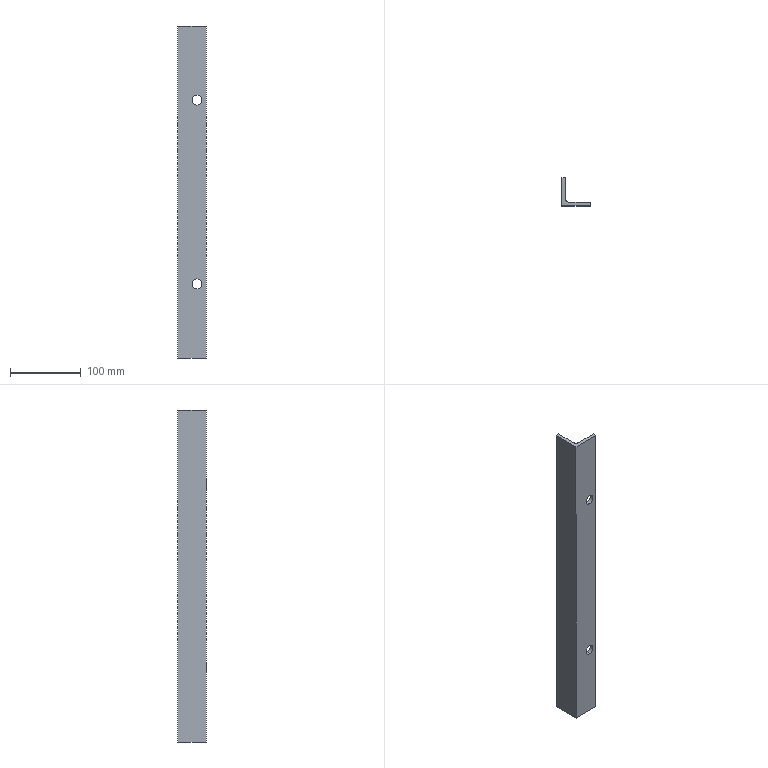Part | NX | features BREP 1 | 1 solid | 13 faces | box 40 x 40 x 470 mm | volume 177232 mm3 | plane 8 | cylinder 5 | commonest cylinder face diameters 14 x4 10 x1
STEP:
#1=CARTESIAN_POINT('',(27.,0.,-137.));
#2=VERTEX_POINT('',#1);
#3=CARTESIAN_POINT('',(27.,0.,-123.));
#4=VERTEX_POINT('',#3);
#5=CARTESIAN_POINT('',(27.,0.,-130.));
#6=DIRECTION('',(0.,1.,0.));
#7=DIRECTION('',(0.,0.,1.));
#8=AXIS2_PLACEMENT_3D('',#5,#6,#7);
#9=CIRCLE('',#8,7.);
#10=EDGE_CURVE('',#2,#4,#9,.T.);
#11=ORIENTED_EDGE('',*,*,#10,.F.);
#12=CARTESIAN_POINT('',(27.,5.,-137.));
#13=VERTEX_POINT('',#12);
#14=CARTESIAN_POINT('',(27.,0.,-137.));
#15=DIRECTION('',(0.,1.,0.));
#16=VECTOR('',#15,1000.);
#17=LINE('',#14,#16);
#18=EDGE_CURVE('',#2,#13,#17,.T.);
#19=ORIENTED_EDGE('',*,*,#18,.T.);
#20=CARTESIAN_POINT('',(27.,5.,-123.));
#21=VERTEX_POINT('',#20);
#22=CARTESIAN_POINT('',(27.,5.,-130.));
#23=DIRECTION('',(0.,1.,0.));
#24=DIRECTION('',(0.,0.,1.));
#25=AXIS2_PLACEMENT_3D('',#22,#23,#24);
#26=CIRCLE('',#25,7.);
#27=EDGE_CURVE('',#13,#21,#26,.T.);
#28=ORIENTED_EDGE('',*,*,#27,.T.);
#29=CARTESIAN_POINT('',(27.,0.,-123.));
#30=DIRECTION('',(0.,1.,0.));
#31=VECTOR('',#30,1000.);
#32=LINE('',#29,#31);
#33=EDGE_CURVE('',#4,#21,#32,.T.);
#34=ORIENTED_EDGE('',*,*,#33,.F.);
#35=EDGE_LOOP('',(#11,#19,#28,#34));
#36=FACE_BOUND('',#35,.T.);
#37=CARTESIAN_POINT('',(27.,0.,-130.));
#38=DIRECTION('',(0.,1.,0.));
#39=DIRECTION('',(0.,0.,-1.));
#40=AXIS2_PLACEMENT_3D('',#37,#38,#39);
#41=CYLINDRICAL_SURFACE('',#40,7.);
#42=ADVANCED_FACE('',(#36),#41,.F.);
#43=CARTESIAN_POINT('',(27.,0.,123.));
#44=VERTEX_POINT('',#43);
#45=CARTESIAN_POINT('',(27.,0.,137.));
#46=VERTEX_POINT('',#45);
#47=CARTESIAN_POINT('',(27.,0.,130.));
#48=DIRECTION('',(0.,1.,0.));
#49=DIRECTION('',(0.,0.,1.));
#50=AXIS2_PLACEMENT_3D('',#47,#48,#49);
#51=CIRCLE('',#50,7.);
#52=EDGE_CURVE('',#44,#46,#51,.T.);
#53=ORIENTED_EDGE('',*,*,#52,.F.);
#54=CARTESIAN_POINT('',(27.,5.,123.));
#55=VERTEX_POINT('',#54);
#56=CARTESIAN_POINT('',(27.,0.,123.));
#57=DIRECTION('',(0.,1.,0.));
#58=VECTOR('',#57,1000.);
#59=LINE('',#56,#58);
#60=EDGE_CURVE('',#44,#55,#59,.T.);
#61=ORIENTED_EDGE('',*,*,#60,.T.);
#62=CARTESIAN_POINT('',(27.,5.,137.));
#63=VERTEX_POINT('',#62);
#64=CARTESIAN_POINT('',(27.,5.,130.));
#65=DIRECTION('',(0.,1.,0.));
#66=DIRECTION('',(0.,0.,1.));
#67=AXIS2_PLACEMENT_3D('',#64,#65,#66);
#68=CIRCLE('',#67,7.);
#69=EDGE_CURVE('',#55,#63,#68,.T.);
#70=ORIENTED_EDGE('',*,*,#69,.T.);
#71=CARTESIAN_POINT('',(27.,0.,137.));
#72=DIRECTION('',(0.,1.,0.));
#73=VECTOR('',#72,1000.);
#74=LINE('',#71,#73);
#75=EDGE_CURVE('',#46,#63,#74,.T.);
#76=ORIENTED_EDGE('',*,*,#75,.F.);
#77=EDGE_LOOP('',(#53,#61,#70,#76));
#78=FACE_BOUND('',#77,.T.);
#79=CARTESIAN_POINT('',(27.,0.,130.));
#80=DIRECTION('',(0.,1.,0.));
#81=DIRECTION('',(0.,0.,-1.));
#82=AXIS2_PLACEMENT_3D('',#79,#80,#81);
#83=CYLINDRICAL_SURFACE('',#82,7.);
#84=ADVANCED_FACE('',(#78),#83,.F.);
#85=CARTESIAN_POINT('',(40.,0.,-235.));
#86=VERTEX_POINT('',#85);
#87=CARTESIAN_POINT('',(40.,5.,-235.));
#88=VERTEX_POINT('',#87);
#89=CARTESIAN_POINT('',(40.,5.,-235.));
#90=DIRECTION('',(0.,1.,0.));
#91=VECTOR('',#90,1000.);
#92=LINE('',#89,#91);
#93=EDGE_CURVE('',#86,#88,#92,.T.);
#94=ORIENTED_EDGE('',*,*,#93,.T.);
#95=CARTESIAN_POINT('',(40.,5.,235.));
#96=VERTEX_POINT('',#95);
#97=CARTESIAN_POINT('',(40.,5.,235.));
#98=DIRECTION('',(0.,0.,-1.));
#99=VECTOR('',#98,1000.);
#100=LINE('',#97,#99);
#101=EDGE_CURVE('',#96,#88,#100,.T.);
#102=ORIENTED_EDGE('',*,*,#101,.F.);
#103=CARTESIAN_POINT('',(40.,0.,235.));
#104=VERTEX_POINT('',#103);
#105=CARTESIAN_POINT('',(40.,5.,235.));
#106=DIRECTION('',(0.,1.,0.));
#107=VECTOR('',#106,1000.);
#108=LINE('',#105,#107);
#109=EDGE_CURVE('',#104,#96,#108,.T.);
#110=ORIENTED_EDGE('',*,*,#109,.F.);
#111=CARTESIAN_POINT('',(40.,0.,235.));
#112=DIRECTION('',(0.,0.,-1.));
#113=VECTOR('',#112,1000.);
#114=LINE('',#111,#113);
#115=EDGE_CURVE('',#104,#86,#114,.T.);
#116=ORIENTED_EDGE('',*,*,#115,.T.);
#117=EDGE_LOOP('',(#94,#102,#110,#116));
#118=FACE_BOUND('',#117,.T.);
#119=CARTESIAN_POINT('',(40.,5.,235.));
#120=DIRECTION('',(-1.,0.,0.));
#121=DIRECTION('',(0.,0.,-1.));
#122=AXIS2_PLACEMENT_3D('',#119,#120,#121);
#123=PLANE('',#122);
#124=ADVANCED_FACE('',(#118),#123,.F.);
#125=CARTESIAN_POINT('',(27.,5.,-130.));
#126=DIRECTION('',(0.,1.,0.));
#127=DIRECTION('',(0.,0.,1.));
#128=AXIS2_PLACEMENT_3D('',#125,#126,#127);
#129=CIRCLE('',#128,7.);
#130=EDGE_CURVE('',#21,#13,#129,.T.);
#131=ORIENTED_EDGE('',*,*,#130,.F.);
#132=ORIENTED_EDGE('',*,*,#27,.F.);
#133=EDGE_LOOP('',(#131,#132));
#134=FACE_BOUND('',#133,.T.);
#135=CARTESIAN_POINT('',(27.,5.,130.));
#136=DIRECTION('',(0.,1.,0.));
#137=DIRECTION('',(0.,0.,1.));
#138=AXIS2_PLACEMENT_3D('',#135,#136,#137);
#139=CIRCLE('',#138,7.);
#140=EDGE_CURVE('',#63,#55,#139,.T.);
#141=ORIENTED_EDGE('',*,*,#140,.F.);
#142=ORIENTED_EDGE('',*,*,#69,.F.);
#143=EDGE_LOOP('',(#141,#142));
#144=FACE_BOUND('',#143,.T.);
#145=CARTESIAN_POINT('',(10.,5.,-235.));
#146=VERTEX_POINT('',#145);
#147=CARTESIAN_POINT('',(10.,5.,-235.));
#148=DIRECTION('',(-1.,0.,0.));
#149=VECTOR('',#148,1000.);
#150=LINE('',#147,#149);
#151=EDGE_CURVE('',#88,#146,#150,.T.);
#152=ORIENTED_EDGE('',*,*,#151,.T.);
#153=CARTESIAN_POINT('',(10.,5.,235.));
#154=VERTEX_POINT('',#153);
#155=CARTESIAN_POINT('',(10.,5.,235.));
#156=DIRECTION('',(0.,0.,-1.));
#157=VECTOR('',#156,1000.);
#158=LINE('',#155,#157);
#159=EDGE_CURVE('',#154,#146,#158,.T.);
#160=ORIENTED_EDGE('',*,*,#159,.F.);
#161=CARTESIAN_POINT('',(10.,5.,235.));
#162=DIRECTION('',(-1.,0.,0.));
#163=VECTOR('',#162,1000.);
#164=LINE('',#161,#163);
#165=EDGE_CURVE('',#96,#154,#164,.T.);
#166=ORIENTED_EDGE('',*,*,#165,.F.);
#167=ORIENTED_EDGE('',*,*,#101,.T.);
#168=EDGE_LOOP('',(#152,#160,#166,#167));
#169=FACE_BOUND('',#168,.T.);
#170=CARTESIAN_POINT('',(10.,5.,235.));
#171=DIRECTION('',(0.,-1.,0.));
#172=DIRECTION('',(0.,0.,1.));
#173=AXIS2_PLACEMENT_3D('',#170,#171,#172);
#174=PLANE('',#173);
#175=ADVANCED_FACE('',(#134,#144,#169),#174,.F.);
#176=CARTESIAN_POINT('',(5.,10.,-235.));
#177=VERTEX_POINT('',#176);
#178=CARTESIAN_POINT('',(10.,10.,-235.));
#179=DIRECTION('',(0.,0.,-1.));
#180=DIRECTION('',(1.,0.,0.));
#181=AXIS2_PLACEMENT_3D('',#178,#179,#180);
#182=CIRCLE('',#181,5.);
#183=EDGE_CURVE('',#146,#177,#182,.T.);
#184=ORIENTED_EDGE('',*,*,#183,.T.);
#185=CARTESIAN_POINT('',(5.,10.,235.));
#186=VERTEX_POINT('',#185);
#187=CARTESIAN_POINT('',(5.,10.,235.));
#188=DIRECTION('',(0.,0.,-1.));
#189=VECTOR('',#188,1000.);
#190=LINE('',#187,#189);
#191=EDGE_CURVE('',#186,#177,#190,.T.);
#192=ORIENTED_EDGE('',*,*,#191,.F.);
#193=CARTESIAN_POINT('',(10.,10.,235.));
#194=DIRECTION('',(0.,0.,-1.));
#195=DIRECTION('',(1.,0.,0.));
#196=AXIS2_PLACEMENT_3D('',#193,#194,#195);
#197=CIRCLE('',#196,5.);
#198=EDGE_CURVE('',#154,#186,#197,.T.);
#199=ORIENTED_EDGE('',*,*,#198,.F.);
#200=ORIENTED_EDGE('',*,*,#159,.T.);
#201=EDGE_LOOP('',(#184,#192,#199,#200));
#202=FACE_BOUND('',#201,.T.);
#203=CARTESIAN_POINT('',(10.,10.,235.));
#204=DIRECTION('',(0.,0.,-1.));
#205=DIRECTION('',(1.,0.,0.));
#206=AXIS2_PLACEMENT_3D('',#203,#204,#205);
#207=CYLINDRICAL_SURFACE('',#206,5.);
#208=ADVANCED_FACE('',(#202),#207,.F.);
#209=CARTESIAN_POINT('',(5.,40.,-235.));
#210=VERTEX_POINT('',#209);
#211=CARTESIAN_POINT('',(5.,40.,-235.));
#212=DIRECTION('',(0.,1.,0.));
#213=VECTOR('',#212,1000.);
#214=LINE('',#211,#213);
#215=EDGE_CURVE('',#177,#210,#214,.T.);
#216=ORIENTED_EDGE('',*,*,#215,.T.);
#217=CARTESIAN_POINT('',(5.,40.,235.));
#218=VERTEX_POINT('',#217);
#219=CARTESIAN_POINT('',(5.,40.,235.));
#220=DIRECTION('',(0.,0.,-1.));
#221=VECTOR('',#220,1000.);
#222=LINE('',#219,#221);
#223=EDGE_CURVE('',#218,#210,#222,.T.);
#224=ORIENTED_EDGE('',*,*,#223,.F.);
#225=CARTESIAN_POINT('',(5.,40.,235.));
#226=DIRECTION('',(0.,1.,0.));
#227=VECTOR('',#226,1000.);
#228=LINE('',#225,#227);
#229=EDGE_CURVE('',#186,#218,#228,.T.);
#230=ORIENTED_EDGE('',*,*,#229,.F.);
#231=ORIENTED_EDGE('',*,*,#191,.T.);
#232=EDGE_LOOP('',(#216,#224,#230,#231));
#233=FACE_BOUND('',#232,.T.);
#234=CARTESIAN_POINT('',(5.,40.,235.));
#235=DIRECTION('',(-1.,0.,0.));
#236=DIRECTION('',(0.,0.,-1.));
#237=AXIS2_PLACEMENT_3D('',#234,#235,#236);
#238=PLANE('',#237);
#239=ADVANCED_FACE('',(#233),#238,.F.);
#240=CARTESIAN_POINT('',(0.,40.,-235.));
#241=VERTEX_POINT('',#240);
#242=CARTESIAN_POINT('',(0.,40.,-235.));
#243=DIRECTION('',(-1.,0.,0.));
#244=VECTOR('',#243,1000.);
#245=LINE('',#242,#244);
#246=EDGE_CURVE('',#210,#241,#245,.T.);
#247=ORIENTED_EDGE('',*,*,#246,.T.);
#248=CARTESIAN_POINT('',(0.,40.,235.));
#249=VERTEX_POINT('',#248);
#250=CARTESIAN_POINT('',(0.,40.,235.));
#251=DIRECTION('',(0.,0.,-1.));
#252=VECTOR('',#251,1000.);
#253=LINE('',#250,#252);
#254=EDGE_CURVE('',#249,#241,#253,.T.);
#255=ORIENTED_EDGE('',*,*,#254,.F.);
#256=CARTESIAN_POINT('',(0.,40.,235.));
#257=DIRECTION('',(-1.,0.,0.));
#258=VECTOR('',#257,1000.);
#259=LINE('',#256,#258);
#260=EDGE_CURVE('',#218,#249,#259,.T.);
#261=ORIENTED_EDGE('',*,*,#260,.F.);
#262=ORIENTED_EDGE('',*,*,#223,.T.);
#263=EDGE_LOOP('',(#247,#255,#261,#262));
#264=FACE_BOUND('',#263,.T.);
#265=CARTESIAN_POINT('',(0.,40.,235.));
#266=DIRECTION('',(0.,-1.,0.));
#267=DIRECTION('',(0.,0.,1.));
#268=AXIS2_PLACEMENT_3D('',#265,#266,#267);
#269=PLANE('',#268);
#270=ADVANCED_FACE('',(#264),#269,.F.);
#271=CARTESIAN_POINT('',(0.,0.,-235.));
#272=VERTEX_POINT('',#271);
#273=CARTESIAN_POINT('',(0.,0.,-235.));
#274=DIRECTION('',(0.,-1.,0.));
#275=VECTOR('',#274,1000.);
#276=LINE('',#273,#275);
#277=EDGE_CURVE('',#241,#272,#276,.T.);
#278=ORIENTED_EDGE('',*,*,#277,.T.);
#279=CARTESIAN_POINT('',(0.,0.,235.));
#280=VERTEX_POINT('',#279);
#281=CARTESIAN_POINT('',(0.,0.,235.));
#282=DIRECTION('',(0.,0.,-1.));
#283=VECTOR('',#282,1000.);
#284=LINE('',#281,#283);
#285=EDGE_CURVE('',#280,#272,#284,.T.);
#286=ORIENTED_EDGE('',*,*,#285,.F.);
#287=CARTESIAN_POINT('',(0.,0.,235.));
#288=DIRECTION('',(0.,-1.,0.));
#289=VECTOR('',#288,1000.);
#290=LINE('',#287,#289);
#291=EDGE_CURVE('',#249,#280,#290,.T.);
#292=ORIENTED_EDGE('',*,*,#291,.F.);
#293=ORIENTED_EDGE('',*,*,#254,.T.);
#294=EDGE_LOOP('',(#278,#286,#292,#293));
#295=FACE_BOUND('',#294,.T.);
#296=CARTESIAN_POINT('',(0.,0.,235.));
#297=DIRECTION('',(1.,0.,0.));
#298=DIRECTION('',(0.,0.,1.));
#299=AXIS2_PLACEMENT_3D('',#296,#297,#298);
#300=PLANE('',#299);
#301=ADVANCED_FACE('',(#295),#300,.F.);
#302=CARTESIAN_POINT('',(27.,0.,-130.));
#303=DIRECTION('',(0.,1.,0.));
#304=DIRECTION('',(0.,0.,1.));
#305=AXIS2_PLACEMENT_3D('',#302,#303,#304);
#306=CIRCLE('',#305,7.);
#307=EDGE_CURVE('',#4,#2,#306,.T.);
#308=ORIENTED_EDGE('',*,*,#307,.T.);
#309=ORIENTED_EDGE('',*,*,#10,.T.);
#310=EDGE_LOOP('',(#308,#309));
#311=FACE_BOUND('',#310,.T.);
#312=CARTESIAN_POINT('',(27.,0.,130.));
#313=DIRECTION('',(0.,1.,0.));
#314=DIRECTION('',(0.,0.,1.));
#315=AXIS2_PLACEMENT_3D('',#312,#313,#314);
#316=CIRCLE('',#315,7.);
#317=EDGE_CURVE('',#46,#44,#316,.T.);
#318=ORIENTED_EDGE('',*,*,#317,.T.);
#319=ORIENTED_EDGE('',*,*,#52,.T.);
#320=EDGE_LOOP('',(#318,#319));
#321=FACE_BOUND('',#320,.T.);
#322=CARTESIAN_POINT('',(40.,0.,-235.));
#323=DIRECTION('',(1.,0.,0.));
#324=VECTOR('',#323,1000.);
#325=LINE('',#322,#324);
#326=EDGE_CURVE('',#272,#86,#325,.T.);
#327=ORIENTED_EDGE('',*,*,#326,.T.);
#328=ORIENTED_EDGE('',*,*,#115,.F.);
#329=CARTESIAN_POINT('',(40.,0.,235.));
#330=DIRECTION('',(1.,0.,0.));
#331=VECTOR('',#330,1000.);
#332=LINE('',#329,#331);
#333=EDGE_CURVE('',#280,#104,#332,.T.);
#334=ORIENTED_EDGE('',*,*,#333,.F.);
#335=ORIENTED_EDGE('',*,*,#285,.T.);
#336=EDGE_LOOP('',(#327,#328,#334,#335));
#337=FACE_BOUND('',#336,.T.);
#338=CARTESIAN_POINT('',(40.,0.,235.));
#339=DIRECTION('',(0.,1.,0.));
#340=DIRECTION('',(0.,0.,-1.));
#341=AXIS2_PLACEMENT_3D('',#338,#339,#340);
#342=PLANE('',#341);
#343=ADVANCED_FACE('',(#311,#321,#337),#342,.F.);
#344=ORIENTED_EDGE('',*,*,#109,.T.);
#345=ORIENTED_EDGE('',*,*,#165,.T.);
#346=ORIENTED_EDGE('',*,*,#198,.T.);
#347=ORIENTED_EDGE('',*,*,#229,.T.);
#348=ORIENTED_EDGE('',*,*,#260,.T.);
#349=ORIENTED_EDGE('',*,*,#291,.T.);
#350=ORIENTED_EDGE('',*,*,#333,.T.);
#351=EDGE_LOOP('',(#344,#345,#346,#347,#348,#349,#350));
#352=FACE_BOUND('',#351,.T.);
#353=CARTESIAN_POINT('',(10.,10.,235.));
#354=DIRECTION('',(0.,0.,1.));
#355=DIRECTION('',(-1.,0.,0.));
#356=AXIS2_PLACEMENT_3D('',#353,#354,#355);
#357=PLANE('',#356);
#358=ADVANCED_FACE('',(#352),#357,.T.);
#359=ORIENTED_EDGE('',*,*,#93,.F.);
#360=ORIENTED_EDGE('',*,*,#326,.F.);
#361=ORIENTED_EDGE('',*,*,#277,.F.);
#362=ORIENTED_EDGE('',*,*,#246,.F.);
#363=ORIENTED_EDGE('',*,*,#215,.F.);
#364=ORIENTED_EDGE('',*,*,#183,.F.);
#365=ORIENTED_EDGE('',*,*,#151,.F.);
#366=EDGE_LOOP('',(#359,#360,#361,#362,#363,#364,#365));
#367=FACE_BOUND('',#366,.T.);
#368=CARTESIAN_POINT('',(10.,10.,-235.));
#369=DIRECTION('',(0.,0.,1.));
#370=DIRECTION('',(-1.,0.,0.));
#371=AXIS2_PLACEMENT_3D('',#368,#369,#370);
#372=PLANE('',#371);
#373=ADVANCED_FACE('',(#367),#372,.F.);
#374=ORIENTED_EDGE('',*,*,#60,.F.);
#375=ORIENTED_EDGE('',*,*,#317,.F.);
#376=ORIENTED_EDGE('',*,*,#75,.T.);
#377=ORIENTED_EDGE('',*,*,#140,.T.);
#378=EDGE_LOOP('',(#374,#375,#376,#377));
#379=FACE_BOUND('',#378,.T.);
#380=CARTESIAN_POINT('',(27.,0.,130.));
#381=DIRECTION('',(0.,1.,0.));
#382=DIRECTION('',(0.,0.,-1.));
#383=AXIS2_PLACEMENT_3D('',#380,#381,#382);
#384=CYLINDRICAL_SURFACE('',#383,7.);
#385=ADVANCED_FACE('',(#379),#384,.F.);
#386=ORIENTED_EDGE('',*,*,#18,.F.);
#387=ORIENTED_EDGE('',*,*,#307,.F.);
#388=ORIENTED_EDGE('',*,*,#33,.T.);
#389=ORIENTED_EDGE('',*,*,#130,.T.);
#390=EDGE_LOOP('',(#386,#387,#388,#389));
#391=FACE_BOUND('',#390,.T.);
#392=CARTESIAN_POINT('',(27.,0.,-130.));
#393=DIRECTION('',(0.,1.,0.));
#394=DIRECTION('',(0.,0.,-1.));
#395=AXIS2_PLACEMENT_3D('',#392,#393,#394);
#396=CYLINDRICAL_SURFACE('',#395,7.);
#397=ADVANCED_FACE('',(#391),#396,.F.);
#398=CLOSED_SHELL('',(#42,#84,#124,#175,#208,#239,#270,#301,#343,#358,#373,#385,#397));
#399=MANIFOLD_SOLID_BREP('',#398);
#400=(LENGTH_UNIT()NAMED_UNIT(*)SI_UNIT(.MILLI.,.METRE.));
#401=UNCERTAINTY_MEASURE_WITH_UNIT(LENGTH_MEASURE(0.00001),#400,'','');
#402=(NAMED_UNIT(*)PLANE_ANGLE_UNIT()SI_UNIT($,.RADIAN.));
#403=(NAMED_UNIT(*)SI_UNIT($,.STERADIAN.)SOLID_ANGLE_UNIT());
#404=(GEOMETRIC_REPRESENTATION_CONTEXT(3)GLOBAL_UNCERTAINTY_ASSIGNED_CONTEXT((#401))GLOBAL_UNIT_ASSIGNED_CONTEXT((#400,#402,#403))REPRESENTATION_CONTEXT('',''));
#405=ADVANCED_BREP_SHAPE_REPRESENTATION('',(#399),#404);